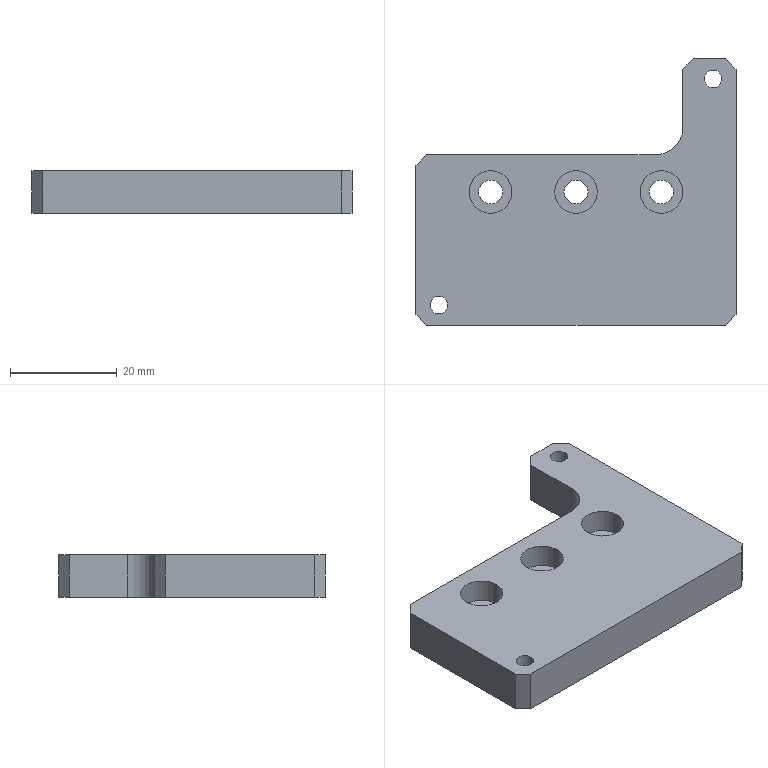Part | SolidWorks | features Chamfer 2, HoleWzd 2, Extrusion 1, Fillet 1, ICE 1 | 1 solid | 33 faces | box 60 x 50 x 8 mm | volume 15791 mm3 | cylinder 17 | plane 16 | commonest cylinder face diameters 4.5 x6 8 x6 3.3 x4 10 x1
STEP:
#1=CARTESIAN_POINT('',(2.65,3.8,0.));
#2=VERTEX_POINT('',#1);
#3=CARTESIAN_POINT('',(5.95,3.8,0.));
#4=VERTEX_POINT('',#3);
#5=CARTESIAN_POINT('',(4.3,3.8,0.));
#6=DIRECTION('',(0.,0.,1.));
#7=DIRECTION('',(1.,0.,0.));
#8=AXIS2_PLACEMENT_3D('',#5,#6,#7);
#9=CIRCLE('',#8,1.65);
#10=EDGE_CURVE('',#2,#4,#9,.T.);
#11=ORIENTED_EDGE('',*,*,#10,.F.);
#12=CARTESIAN_POINT('',(2.65,3.8,8.));
#13=VERTEX_POINT('',#12);
#14=CARTESIAN_POINT('',(2.65,3.8,8.));
#15=DIRECTION('',(0.,0.,1.));
#16=VECTOR('',#15,1000.);
#17=LINE('',#14,#16);
#18=EDGE_CURVE('',#2,#13,#17,.T.);
#19=ORIENTED_EDGE('',*,*,#18,.T.);
#20=CARTESIAN_POINT('',(5.95,3.8,8.));
#21=VERTEX_POINT('',#20);
#22=CARTESIAN_POINT('',(4.3,3.8,8.));
#23=DIRECTION('',(0.,0.,1.));
#24=DIRECTION('',(1.,0.,0.));
#25=AXIS2_PLACEMENT_3D('',#22,#23,#24);
#26=CIRCLE('',#25,1.65);
#27=EDGE_CURVE('',#13,#21,#26,.T.);
#28=ORIENTED_EDGE('',*,*,#27,.T.);
#29=CARTESIAN_POINT('',(5.95,3.8,8.));
#30=DIRECTION('',(0.,0.,1.));
#31=VECTOR('',#30,1000.);
#32=LINE('',#29,#31);
#33=EDGE_CURVE('',#4,#21,#32,.T.);
#34=ORIENTED_EDGE('',*,*,#33,.F.);
#35=EDGE_LOOP('',(#11,#19,#28,#34));
#36=FACE_OUTER_BOUND('',#35,.T.);
#37=CARTESIAN_POINT('',(4.3,3.8,8.));
#38=DIRECTION('',(0.,0.,1.));
#39=DIRECTION('',(1.,0.,0.));
#40=AXIS2_PLACEMENT_3D('',#37,#38,#39);
#41=CYLINDRICAL_SURFACE('',#40,1.65);
#42=ADVANCED_FACE('',(#36),#41,.F.);
#43=CARTESIAN_POINT('',(54.05,46.2,0.));
#44=VERTEX_POINT('',#43);
#45=CARTESIAN_POINT('',(57.35,46.2,0.));
#46=VERTEX_POINT('',#45);
#47=CARTESIAN_POINT('',(55.7,46.2,0.));
#48=DIRECTION('',(0.,0.,1.));
#49=DIRECTION('',(1.,0.,0.));
#50=AXIS2_PLACEMENT_3D('',#47,#48,#49);
#51=CIRCLE('',#50,1.65);
#52=EDGE_CURVE('',#44,#46,#51,.T.);
#53=ORIENTED_EDGE('',*,*,#52,.F.);
#54=CARTESIAN_POINT('',(54.05,46.2,8.));
#55=VERTEX_POINT('',#54);
#56=CARTESIAN_POINT('',(54.05,46.2,8.));
#57=DIRECTION('',(0.,0.,1.));
#58=VECTOR('',#57,1000.);
#59=LINE('',#56,#58);
#60=EDGE_CURVE('',#44,#55,#59,.T.);
#61=ORIENTED_EDGE('',*,*,#60,.T.);
#62=CARTESIAN_POINT('',(57.35,46.2,8.));
#63=VERTEX_POINT('',#62);
#64=CARTESIAN_POINT('',(55.7,46.2,8.));
#65=DIRECTION('',(0.,0.,1.));
#66=DIRECTION('',(1.,0.,0.));
#67=AXIS2_PLACEMENT_3D('',#64,#65,#66);
#68=CIRCLE('',#67,1.65);
#69=EDGE_CURVE('',#55,#63,#68,.T.);
#70=ORIENTED_EDGE('',*,*,#69,.T.);
#71=CARTESIAN_POINT('',(57.35,46.2,8.));
#72=DIRECTION('',(0.,0.,1.));
#73=VECTOR('',#72,1000.);
#74=LINE('',#71,#73);
#75=EDGE_CURVE('',#46,#63,#74,.T.);
#76=ORIENTED_EDGE('',*,*,#75,.F.);
#77=EDGE_LOOP('',(#53,#61,#70,#76));
#78=FACE_OUTER_BOUND('',#77,.T.);
#79=CARTESIAN_POINT('',(55.7,46.2,8.));
#80=DIRECTION('',(0.,0.,1.));
#81=DIRECTION('',(1.,0.,0.));
#82=AXIS2_PLACEMENT_3D('',#79,#80,#81);
#83=CYLINDRICAL_SURFACE('',#82,1.65);
#84=ADVANCED_FACE('',(#78),#83,.F.);
#85=CARTESIAN_POINT('',(26.,25.,3.6));
#86=VERTEX_POINT('',#85);
#87=CARTESIAN_POINT('',(34.,25.,3.6));
#88=VERTEX_POINT('',#87);
#89=CARTESIAN_POINT('',(30.,25.,3.6));
#90=DIRECTION('',(0.,0.,1.));
#91=DIRECTION('',(1.,0.,0.));
#92=AXIS2_PLACEMENT_3D('',#89,#90,#91);
#93=CIRCLE('',#92,4.);
#94=EDGE_CURVE('',#86,#88,#93,.T.);
#95=ORIENTED_EDGE('',*,*,#94,.F.);
#96=CARTESIAN_POINT('',(26.,25.,8.));
#97=VERTEX_POINT('',#96);
#98=CARTESIAN_POINT('',(26.,25.,8.));
#99=DIRECTION('',(0.,0.,1.));
#100=VECTOR('',#99,1000.);
#101=LINE('',#98,#100);
#102=EDGE_CURVE('',#86,#97,#101,.T.);
#103=ORIENTED_EDGE('',*,*,#102,.T.);
#104=CARTESIAN_POINT('',(34.,25.,8.));
#105=VERTEX_POINT('',#104);
#106=CARTESIAN_POINT('',(30.,25.,8.));
#107=DIRECTION('',(0.,0.,1.));
#108=DIRECTION('',(1.,0.,0.));
#109=AXIS2_PLACEMENT_3D('',#106,#107,#108);
#110=CIRCLE('',#109,4.);
#111=EDGE_CURVE('',#97,#105,#110,.T.);
#112=ORIENTED_EDGE('',*,*,#111,.T.);
#113=CARTESIAN_POINT('',(34.,25.,8.));
#114=DIRECTION('',(0.,0.,1.));
#115=VECTOR('',#114,1000.);
#116=LINE('',#113,#115);
#117=EDGE_CURVE('',#88,#105,#116,.T.);
#118=ORIENTED_EDGE('',*,*,#117,.F.);
#119=EDGE_LOOP('',(#95,#103,#112,#118));
#120=FACE_OUTER_BOUND('',#119,.T.);
#121=CARTESIAN_POINT('',(30.,25.,8.));
#122=DIRECTION('',(0.,0.,1.));
#123=DIRECTION('',(1.,0.,0.));
#124=AXIS2_PLACEMENT_3D('',#121,#122,#123);
#125=CYLINDRICAL_SURFACE('',#124,4.);
#126=ADVANCED_FACE('',(#120),#125,.F.);
#127=CARTESIAN_POINT('',(27.75,25.,0.));
#128=VERTEX_POINT('',#127);
#129=CARTESIAN_POINT('',(32.25,25.,0.));
#130=VERTEX_POINT('',#129);
#131=CARTESIAN_POINT('',(30.,25.,0.));
#132=DIRECTION('',(0.,0.,1.));
#133=DIRECTION('',(1.,0.,0.));
#134=AXIS2_PLACEMENT_3D('',#131,#132,#133);
#135=CIRCLE('',#134,2.25);
#136=EDGE_CURVE('',#128,#130,#135,.T.);
#137=ORIENTED_EDGE('',*,*,#136,.F.);
#138=CARTESIAN_POINT('',(27.75,25.,3.6));
#139=VERTEX_POINT('',#138);
#140=CARTESIAN_POINT('',(27.75,25.,8.));
#141=DIRECTION('',(0.,0.,1.));
#142=VECTOR('',#141,1000.);
#143=LINE('',#140,#142);
#144=EDGE_CURVE('',#128,#139,#143,.T.);
#145=ORIENTED_EDGE('',*,*,#144,.T.);
#146=CARTESIAN_POINT('',(32.25,25.,3.6));
#147=VERTEX_POINT('',#146);
#148=CARTESIAN_POINT('',(30.,25.,3.6));
#149=DIRECTION('',(0.,0.,1.));
#150=DIRECTION('',(1.,0.,0.));
#151=AXIS2_PLACEMENT_3D('',#148,#149,#150);
#152=CIRCLE('',#151,2.25);
#153=EDGE_CURVE('',#139,#147,#152,.T.);
#154=ORIENTED_EDGE('',*,*,#153,.T.);
#155=CARTESIAN_POINT('',(32.25,25.,8.));
#156=DIRECTION('',(0.,0.,1.));
#157=VECTOR('',#156,1000.);
#158=LINE('',#155,#157);
#159=EDGE_CURVE('',#130,#147,#158,.T.);
#160=ORIENTED_EDGE('',*,*,#159,.F.);
#161=EDGE_LOOP('',(#137,#145,#154,#160));
#162=FACE_OUTER_BOUND('',#161,.T.);
#163=CARTESIAN_POINT('',(30.,25.,8.));
#164=DIRECTION('',(0.,0.,1.));
#165=DIRECTION('',(1.,0.,0.));
#166=AXIS2_PLACEMENT_3D('',#163,#164,#165);
#167=CYLINDRICAL_SURFACE('',#166,2.25);
#168=ADVANCED_FACE('',(#162),#167,.F.);
#169=CARTESIAN_POINT('',(10.,25.,3.6));
#170=VERTEX_POINT('',#169);
#171=CARTESIAN_POINT('',(18.,25.,3.6));
#172=VERTEX_POINT('',#171);
#173=CARTESIAN_POINT('',(14.,25.,3.6));
#174=DIRECTION('',(0.,0.,1.));
#175=DIRECTION('',(1.,0.,0.));
#176=AXIS2_PLACEMENT_3D('',#173,#174,#175);
#177=CIRCLE('',#176,4.);
#178=EDGE_CURVE('',#170,#172,#177,.T.);
#179=ORIENTED_EDGE('',*,*,#178,.F.);
#180=CARTESIAN_POINT('',(10.,25.,8.));
#181=VERTEX_POINT('',#180);
#182=CARTESIAN_POINT('',(10.,25.,8.));
#183=DIRECTION('',(0.,0.,1.));
#184=VECTOR('',#183,1000.);
#185=LINE('',#182,#184);
#186=EDGE_CURVE('',#170,#181,#185,.T.);
#187=ORIENTED_EDGE('',*,*,#186,.T.);
#188=CARTESIAN_POINT('',(18.,25.,8.));
#189=VERTEX_POINT('',#188);
#190=CARTESIAN_POINT('',(14.,25.,8.));
#191=DIRECTION('',(0.,0.,1.));
#192=DIRECTION('',(1.,0.,0.));
#193=AXIS2_PLACEMENT_3D('',#190,#191,#192);
#194=CIRCLE('',#193,4.);
#195=EDGE_CURVE('',#181,#189,#194,.T.);
#196=ORIENTED_EDGE('',*,*,#195,.T.);
#197=CARTESIAN_POINT('',(18.,25.,8.));
#198=DIRECTION('',(0.,0.,1.));
#199=VECTOR('',#198,1000.);
#200=LINE('',#197,#199);
#201=EDGE_CURVE('',#172,#189,#200,.T.);
#202=ORIENTED_EDGE('',*,*,#201,.F.);
#203=EDGE_LOOP('',(#179,#187,#196,#202));
#204=FACE_OUTER_BOUND('',#203,.T.);
#205=CARTESIAN_POINT('',(14.,25.,8.));
#206=DIRECTION('',(0.,0.,1.));
#207=DIRECTION('',(1.,0.,0.));
#208=AXIS2_PLACEMENT_3D('',#205,#206,#207);
#209=CYLINDRICAL_SURFACE('',#208,4.);
#210=ADVANCED_FACE('',(#204),#209,.F.);
#211=CARTESIAN_POINT('',(11.75,25.,0.));
#212=VERTEX_POINT('',#211);
#213=CARTESIAN_POINT('',(16.25,25.,0.));
#214=VERTEX_POINT('',#213);
#215=CARTESIAN_POINT('',(14.,25.,0.));
#216=DIRECTION('',(0.,0.,1.));
#217=DIRECTION('',(1.,0.,0.));
#218=AXIS2_PLACEMENT_3D('',#215,#216,#217);
#219=CIRCLE('',#218,2.25);
#220=EDGE_CURVE('',#212,#214,#219,.T.);
#221=ORIENTED_EDGE('',*,*,#220,.F.);
#222=CARTESIAN_POINT('',(11.75,25.,3.6));
#223=VERTEX_POINT('',#222);
#224=CARTESIAN_POINT('',(11.75,25.,8.));
#225=DIRECTION('',(0.,0.,1.));
#226=VECTOR('',#225,1000.);
#227=LINE('',#224,#226);
#228=EDGE_CURVE('',#212,#223,#227,.T.);
#229=ORIENTED_EDGE('',*,*,#228,.T.);
#230=CARTESIAN_POINT('',(16.25,25.,3.6));
#231=VERTEX_POINT('',#230);
#232=CARTESIAN_POINT('',(14.,25.,3.6));
#233=DIRECTION('',(0.,0.,1.));
#234=DIRECTION('',(1.,0.,0.));
#235=AXIS2_PLACEMENT_3D('',#232,#233,#234);
#236=CIRCLE('',#235,2.25);
#237=EDGE_CURVE('',#223,#231,#236,.T.);
#238=ORIENTED_EDGE('',*,*,#237,.T.);
#239=CARTESIAN_POINT('',(16.25,25.,8.));
#240=DIRECTION('',(0.,0.,1.));
#241=VECTOR('',#240,1000.);
#242=LINE('',#239,#241);
#243=EDGE_CURVE('',#214,#231,#242,.T.);
#244=ORIENTED_EDGE('',*,*,#243,.F.);
#245=EDGE_LOOP('',(#221,#229,#238,#244));
#246=FACE_OUTER_BOUND('',#245,.T.);
#247=CARTESIAN_POINT('',(14.,25.,8.));
#248=DIRECTION('',(0.,0.,1.));
#249=DIRECTION('',(1.,0.,0.));
#250=AXIS2_PLACEMENT_3D('',#247,#248,#249);
#251=CYLINDRICAL_SURFACE('',#250,2.25);
#252=ADVANCED_FACE('',(#246),#251,.F.);
#253=CARTESIAN_POINT('',(42.,25.,3.6));
#254=VERTEX_POINT('',#253);
#255=CARTESIAN_POINT('',(50.,25.,3.6));
#256=VERTEX_POINT('',#255);
#257=CARTESIAN_POINT('',(46.,25.,3.6));
#258=DIRECTION('',(0.,0.,1.));
#259=DIRECTION('',(1.,0.,0.));
#260=AXIS2_PLACEMENT_3D('',#257,#258,#259);
#261=CIRCLE('',#260,4.);
#262=EDGE_CURVE('',#254,#256,#261,.T.);
#263=ORIENTED_EDGE('',*,*,#262,.F.);
#264=CARTESIAN_POINT('',(42.,25.,8.));
#265=VERTEX_POINT('',#264);
#266=CARTESIAN_POINT('',(42.,25.,8.));
#267=DIRECTION('',(0.,0.,1.));
#268=VECTOR('',#267,1000.);
#269=LINE('',#266,#268);
#270=EDGE_CURVE('',#254,#265,#269,.T.);
#271=ORIENTED_EDGE('',*,*,#270,.T.);
#272=CARTESIAN_POINT('',(50.,25.,8.));
#273=VERTEX_POINT('',#272);
#274=CARTESIAN_POINT('',(46.,25.,8.));
#275=DIRECTION('',(0.,0.,1.));
#276=DIRECTION('',(1.,0.,0.));
#277=AXIS2_PLACEMENT_3D('',#274,#275,#276);
#278=CIRCLE('',#277,4.);
#279=EDGE_CURVE('',#265,#273,#278,.T.);
#280=ORIENTED_EDGE('',*,*,#279,.T.);
#281=CARTESIAN_POINT('',(50.,25.,8.));
#282=DIRECTION('',(0.,0.,1.));
#283=VECTOR('',#282,1000.);
#284=LINE('',#281,#283);
#285=EDGE_CURVE('',#256,#273,#284,.T.);
#286=ORIENTED_EDGE('',*,*,#285,.F.);
#287=EDGE_LOOP('',(#263,#271,#280,#286));
#288=FACE_OUTER_BOUND('',#287,.T.);
#289=CARTESIAN_POINT('',(46.,25.,8.));
#290=DIRECTION('',(0.,0.,1.));
#291=DIRECTION('',(1.,0.,0.));
#292=AXIS2_PLACEMENT_3D('',#289,#290,#291);
#293=CYLINDRICAL_SURFACE('',#292,4.);
#294=ADVANCED_FACE('',(#288),#293,.F.);
#295=CARTESIAN_POINT('',(43.75,25.,0.));
#296=VERTEX_POINT('',#295);
#297=CARTESIAN_POINT('',(48.25,25.,0.));
#298=VERTEX_POINT('',#297);
#299=CARTESIAN_POINT('',(46.,25.,0.));
#300=DIRECTION('',(0.,0.,1.));
#301=DIRECTION('',(1.,0.,0.));
#302=AXIS2_PLACEMENT_3D('',#299,#300,#301);
#303=CIRCLE('',#302,2.25);
#304=EDGE_CURVE('',#296,#298,#303,.T.);
#305=ORIENTED_EDGE('',*,*,#304,.F.);
#306=CARTESIAN_POINT('',(43.75,25.,3.6));
#307=VERTEX_POINT('',#306);
#308=CARTESIAN_POINT('',(43.75,25.,8.));
#309=DIRECTION('',(0.,0.,1.));
#310=VECTOR('',#309,1000.);
#311=LINE('',#308,#310);
#312=EDGE_CURVE('',#296,#307,#311,.T.);
#313=ORIENTED_EDGE('',*,*,#312,.T.);
#314=CARTESIAN_POINT('',(48.25,25.,3.6));
#315=VERTEX_POINT('',#314);
#316=CARTESIAN_POINT('',(46.,25.,3.6));
#317=DIRECTION('',(0.,0.,1.));
#318=DIRECTION('',(1.,0.,0.));
#319=AXIS2_PLACEMENT_3D('',#316,#317,#318);
#320=CIRCLE('',#319,2.25);
#321=EDGE_CURVE('',#307,#315,#320,.T.);
#322=ORIENTED_EDGE('',*,*,#321,.T.);
#323=CARTESIAN_POINT('',(48.25,25.,8.));
#324=DIRECTION('',(0.,0.,1.));
#325=VECTOR('',#324,1000.);
#326=LINE('',#323,#325);
#327=EDGE_CURVE('',#298,#315,#326,.T.);
#328=ORIENTED_EDGE('',*,*,#327,.F.);
#329=EDGE_LOOP('',(#305,#313,#322,#328));
#330=FACE_OUTER_BOUND('',#329,.T.);
#331=CARTESIAN_POINT('',(46.,25.,8.));
#332=DIRECTION('',(0.,0.,1.));
#333=DIRECTION('',(1.,0.,0.));
#334=AXIS2_PLACEMENT_3D('',#331,#332,#333);
#335=CYLINDRICAL_SURFACE('',#334,2.25);
#336=ADVANCED_FACE('',(#330),#335,.F.);
#337=CARTESIAN_POINT('',(0.,30.,8.));
#338=VERTEX_POINT('',#337);
#339=CARTESIAN_POINT('',(0.,2.,8.));
#340=VERTEX_POINT('',#339);
#341=CARTESIAN_POINT('',(0.,0.,8.));
#342=DIRECTION('',(0.,-1.,0.));
#343=VECTOR('',#342,1000.);
#344=LINE('',#341,#343);
#345=EDGE_CURVE('',#338,#340,#344,.T.);
#346=ORIENTED_EDGE('',*,*,#345,.F.);
#347=CARTESIAN_POINT('',(0.,30.,0.));
#348=VERTEX_POINT('',#347);
#349=CARTESIAN_POINT('',(0.,30.,8.));
#350=DIRECTION('',(0.,0.,-1.));
#351=VECTOR('',#350,1000.);
#352=LINE('',#349,#351);
#353=EDGE_CURVE('',#338,#348,#352,.T.);
#354=ORIENTED_EDGE('',*,*,#353,.T.);
#355=CARTESIAN_POINT('',(0.,2.,0.));
#356=VERTEX_POINT('',#355);
#357=CARTESIAN_POINT('',(0.,0.,0.));
#358=DIRECTION('',(0.,-1.,0.));
#359=VECTOR('',#358,1000.);
#360=LINE('',#357,#359);
#361=EDGE_CURVE('',#348,#356,#360,.T.);
#362=ORIENTED_EDGE('',*,*,#361,.T.);
#363=CARTESIAN_POINT('',(0.,2.,8.));
#364=DIRECTION('',(0.,0.,1.));
#365=VECTOR('',#364,1000.);
#366=LINE('',#363,#365);
#367=EDGE_CURVE('',#356,#340,#366,.T.);
#368=ORIENTED_EDGE('',*,*,#367,.T.);
#369=EDGE_LOOP('',(#346,#354,#362,#368));
#370=FACE_OUTER_BOUND('',#369,.T.);
#371=CARTESIAN_POINT('',(0.,0.,8.));
#372=DIRECTION('',(1.,0.,0.));
#373=DIRECTION('',(0.,0.,-1.));
#374=AXIS2_PLACEMENT_3D('',#371,#372,#373);
#375=PLANE('',#374);
#376=ADVANCED_FACE('',(#370),#375,.F.);
#377=CARTESIAN_POINT('',(2.,0.,0.));
#378=VERTEX_POINT('',#377);
#379=CARTESIAN_POINT('',(58.,0.,0.));
#380=VERTEX_POINT('',#379);
#381=CARTESIAN_POINT('',(0.,0.,0.));
#382=DIRECTION('',(1.,0.,0.));
#383=VECTOR('',#382,1000.);
#384=LINE('',#381,#383);
#385=EDGE_CURVE('',#378,#380,#384,.T.);
#386=ORIENTED_EDGE('',*,*,#385,.T.);
#387=CARTESIAN_POINT('',(58.,0.,8.));
#388=VERTEX_POINT('',#387);
#389=CARTESIAN_POINT('',(58.,0.,8.));
#390=DIRECTION('',(0.,0.,1.));
#391=VECTOR('',#390,1000.);
#392=LINE('',#389,#391);
#393=EDGE_CURVE('',#380,#388,#392,.T.);
#394=ORIENTED_EDGE('',*,*,#393,.T.);
#395=CARTESIAN_POINT('',(2.,0.,8.));
#396=VERTEX_POINT('',#395);
#397=CARTESIAN_POINT('',(0.,0.,8.));
#398=DIRECTION('',(1.,0.,0.));
#399=VECTOR('',#398,1000.);
#400=LINE('',#397,#399);
#401=EDGE_CURVE('',#396,#388,#400,.T.);
#402=ORIENTED_EDGE('',*,*,#401,.F.);
#403=CARTESIAN_POINT('',(2.,0.,8.));
#404=DIRECTION('',(0.,0.,-1.));
#405=VECTOR('',#404,1000.);
#406=LINE('',#403,#405);
#407=EDGE_CURVE('',#396,#378,#406,.T.);
#408=ORIENTED_EDGE('',*,*,#407,.T.);
#409=EDGE_LOOP('',(#386,#394,#402,#408));
#410=FACE_OUTER_BOUND('',#409,.T.);
#411=CARTESIAN_POINT('',(0.,0.,8.));
#412=DIRECTION('',(0.,1.,0.));
#413=DIRECTION('',(0.,0.,1.));
#414=AXIS2_PLACEMENT_3D('',#411,#412,#413);
#415=PLANE('',#414);
#416=ADVANCED_FACE('',(#410),#415,.F.);
#417=CARTESIAN_POINT('',(60.,2.,0.));
#418=VERTEX_POINT('',#417);
#419=CARTESIAN_POINT('',(60.,48.,0.));
#420=VERTEX_POINT('',#419);
#421=CARTESIAN_POINT('',(60.,0.,0.));
#422=DIRECTION('',(0.,1.,0.));
#423=VECTOR('',#422,1000.);
#424=LINE('',#421,#423);
#425=EDGE_CURVE('',#418,#420,#424,.T.);
#426=ORIENTED_EDGE('',*,*,#425,.T.);
#427=CARTESIAN_POINT('',(60.,48.,8.));
#428=VERTEX_POINT('',#427);
#429=CARTESIAN_POINT('',(60.,48.,8.));
#430=DIRECTION('',(0.,0.,1.));
#431=VECTOR('',#430,1000.);
#432=LINE('',#429,#431);
#433=EDGE_CURVE('',#420,#428,#432,.T.);
#434=ORIENTED_EDGE('',*,*,#433,.T.);
#435=CARTESIAN_POINT('',(60.,2.,8.));
#436=VERTEX_POINT('',#435);
#437=CARTESIAN_POINT('',(60.,0.,8.));
#438=DIRECTION('',(0.,1.,0.));
#439=VECTOR('',#438,1000.);
#440=LINE('',#437,#439);
#441=EDGE_CURVE('',#436,#428,#440,.T.);
#442=ORIENTED_EDGE('',*,*,#441,.F.);
#443=CARTESIAN_POINT('',(60.,2.,8.));
#444=DIRECTION('',(0.,0.,-1.));
#445=VECTOR('',#444,1000.);
#446=LINE('',#443,#445);
#447=EDGE_CURVE('',#436,#418,#446,.T.);
#448=ORIENTED_EDGE('',*,*,#447,.T.);
#449=EDGE_LOOP('',(#426,#434,#442,#448));
#450=FACE_OUTER_BOUND('',#449,.T.);
#451=CARTESIAN_POINT('',(60.,0.,8.));
#452=DIRECTION('',(-1.,0.,0.));
#453=DIRECTION('',(0.,0.,1.));
#454=AXIS2_PLACEMENT_3D('',#451,#452,#453);
#455=PLANE('',#454);
#456=ADVANCED_FACE('',(#450),#455,.F.);
#457=CARTESIAN_POINT('',(58.,50.,0.));
#458=VERTEX_POINT('',#457);
#459=CARTESIAN_POINT('',(52.,50.,0.));
#460=VERTEX_POINT('',#459);
#461=CARTESIAN_POINT('',(0.,50.,0.));
#462=DIRECTION('',(-1.,0.,0.));
#463=VECTOR('',#462,1000.);
#464=LINE('',#461,#463);
#465=EDGE_CURVE('',#458,#460,#464,.T.);
#466=ORIENTED_EDGE('',*,*,#465,.T.);
#467=CARTESIAN_POINT('',(52.,50.,8.));
#468=VERTEX_POINT('',#467);
#469=CARTESIAN_POINT('',(52.,50.,8.));
#470=DIRECTION('',(0.,0.,1.));
#471=VECTOR('',#470,1000.);
#472=LINE('',#469,#471);
#473=EDGE_CURVE('',#460,#468,#472,.T.);
#474=ORIENTED_EDGE('',*,*,#473,.T.);
#475=CARTESIAN_POINT('',(58.,50.,8.));
#476=VERTEX_POINT('',#475);
#477=CARTESIAN_POINT('',(0.,50.,8.));
#478=DIRECTION('',(-1.,0.,0.));
#479=VECTOR('',#478,1000.);
#480=LINE('',#477,#479);
#481=EDGE_CURVE('',#476,#468,#480,.T.);
#482=ORIENTED_EDGE('',*,*,#481,.F.);
#483=CARTESIAN_POINT('',(58.,50.,8.));
#484=DIRECTION('',(0.,0.,-1.));
#485=VECTOR('',#484,1000.);
#486=LINE('',#483,#485);
#487=EDGE_CURVE('',#476,#458,#486,.T.);
#488=ORIENTED_EDGE('',*,*,#487,.T.);
#489=EDGE_LOOP('',(#466,#474,#482,#488));
#490=FACE_OUTER_BOUND('',#489,.T.);
#491=CARTESIAN_POINT('',(0.,50.,8.));
#492=DIRECTION('',(0.,-1.,0.));
#493=DIRECTION('',(0.,0.,-1.));
#494=AXIS2_PLACEMENT_3D('',#491,#492,#493);
#495=PLANE('',#494);
#496=ADVANCED_FACE('',(#490),#495,.F.);
#497=CARTESIAN_POINT('',(4.3,3.8,8.));
#498=DIRECTION('',(0.,0.,1.));
#499=DIRECTION('',(1.,0.,0.));
#500=AXIS2_PLACEMENT_3D('',#497,#498,#499);
#501=CIRCLE('',#500,1.65);
#502=EDGE_CURVE('',#21,#13,#501,.T.);
#503=ORIENTED_EDGE('',*,*,#502,.F.);
#504=ORIENTED_EDGE('',*,*,#27,.F.);
#505=EDGE_LOOP('',(#503,#504));
#506=FACE_BOUND('',#505,.T.);
#507=CARTESIAN_POINT('',(55.7,46.2,8.));
#508=DIRECTION('',(0.,0.,1.));
#509=DIRECTION('',(1.,0.,0.));
#510=AXIS2_PLACEMENT_3D('',#507,#508,#509);
#511=CIRCLE('',#510,1.65);
#512=EDGE_CURVE('',#63,#55,#511,.T.);
#513=ORIENTED_EDGE('',*,*,#512,.F.);
#514=ORIENTED_EDGE('',*,*,#69,.F.);
#515=EDGE_LOOP('',(#513,#514));
#516=FACE_BOUND('',#515,.T.);
#517=CARTESIAN_POINT('',(30.,25.,8.));
#518=DIRECTION('',(0.,0.,1.));
#519=DIRECTION('',(1.,0.,0.));
#520=AXIS2_PLACEMENT_3D('',#517,#518,#519);
#521=CIRCLE('',#520,4.);
#522=EDGE_CURVE('',#105,#97,#521,.T.);
#523=ORIENTED_EDGE('',*,*,#522,.F.);
#524=ORIENTED_EDGE('',*,*,#111,.F.);
#525=EDGE_LOOP('',(#523,#524));
#526=FACE_BOUND('',#525,.T.);
#527=CARTESIAN_POINT('',(14.,25.,8.));
#528=DIRECTION('',(0.,0.,1.));
#529=DIRECTION('',(1.,0.,0.));
#530=AXIS2_PLACEMENT_3D('',#527,#528,#529);
#531=CIRCLE('',#530,4.);
#532=EDGE_CURVE('',#189,#181,#531,.T.);
#533=ORIENTED_EDGE('',*,*,#532,.F.);
#534=ORIENTED_EDGE('',*,*,#195,.F.);
#535=EDGE_LOOP('',(#533,#534));
#536=FACE_BOUND('',#535,.T.);
#537=CARTESIAN_POINT('',(46.,25.,8.));
#538=DIRECTION('',(0.,0.,1.));
#539=DIRECTION('',(1.,0.,0.));
#540=AXIS2_PLACEMENT_3D('',#537,#538,#539);
#541=CIRCLE('',#540,4.);
#542=EDGE_CURVE('',#273,#265,#541,.T.);
#543=ORIENTED_EDGE('',*,*,#542,.F.);
#544=ORIENTED_EDGE('',*,*,#279,.F.);
#545=EDGE_LOOP('',(#543,#544));
#546=FACE_BOUND('',#545,.T.);
#547=CARTESIAN_POINT('',(50.,48.,8.));
#548=VERTEX_POINT('',#547);
#549=CARTESIAN_POINT('',(50.,37.,8.));
#550=VERTEX_POINT('',#549);
#551=CARTESIAN_POINT('',(50.,32.,8.));
#552=DIRECTION('',(0.,-1.,0.));
#553=VECTOR('',#552,1000.);
#554=LINE('',#551,#553);
#555=EDGE_CURVE('',#548,#550,#554,.T.);
#556=ORIENTED_EDGE('',*,*,#555,.T.);
#557=CARTESIAN_POINT('',(45.,32.,8.));
#558=VERTEX_POINT('',#557);
#559=CARTESIAN_POINT('',(45.,37.,8.));
#560=DIRECTION('',(0.,0.,-1.));
#561=DIRECTION('',(-1.,0.,0.));
#562=AXIS2_PLACEMENT_3D('',#559,#560,#561);
#563=CIRCLE('',#562,5.);
#564=EDGE_CURVE('',#550,#558,#563,.T.);
#565=ORIENTED_EDGE('',*,*,#564,.T.);
#566=CARTESIAN_POINT('',(2.,32.,8.));
#567=VERTEX_POINT('',#566);
#568=CARTESIAN_POINT('',(50.,32.,8.));
#569=DIRECTION('',(-1.,0.,0.));
#570=VECTOR('',#569,1000.);
#571=LINE('',#568,#570);
#572=EDGE_CURVE('',#558,#567,#571,.T.);
#573=ORIENTED_EDGE('',*,*,#572,.T.);
#574=CARTESIAN_POINT('',(0.,30.,8.));
#575=DIRECTION('',(-0.7071,-0.7071,0.));
#576=VECTOR('',#575,1000.);
#577=LINE('',#574,#576);
#578=EDGE_CURVE('',#567,#338,#577,.T.);
#579=ORIENTED_EDGE('',*,*,#578,.T.);
#580=ORIENTED_EDGE('',*,*,#345,.T.);
#581=CARTESIAN_POINT('',(2.,0.,8.));
#582=DIRECTION('',(0.7071,-0.7071,0.));
#583=VECTOR('',#582,1000.);
#584=LINE('',#581,#583);
#585=EDGE_CURVE('',#340,#396,#584,.T.);
#586=ORIENTED_EDGE('',*,*,#585,.T.);
#587=ORIENTED_EDGE('',*,*,#401,.T.);
#588=CARTESIAN_POINT('',(60.,2.,8.));
#589=DIRECTION('',(0.7071,0.7071,0.));
#590=VECTOR('',#589,1000.);
#591=LINE('',#588,#590);
#592=EDGE_CURVE('',#388,#436,#591,.T.);
#593=ORIENTED_EDGE('',*,*,#592,.T.);
#594=ORIENTED_EDGE('',*,*,#441,.T.);
#595=CARTESIAN_POINT('',(58.,50.,8.));
#596=DIRECTION('',(-0.7071,0.7071,0.));
#597=VECTOR('',#596,1000.);
#598=LINE('',#595,#597);
#599=EDGE_CURVE('',#428,#476,#598,.T.);
#600=ORIENTED_EDGE('',*,*,#599,.T.);
#601=ORIENTED_EDGE('',*,*,#481,.T.);
#602=CARTESIAN_POINT('',(50.,48.,8.));
#603=DIRECTION('',(-0.7071,-0.7071,0.));
#604=VECTOR('',#603,1000.);
#605=LINE('',#602,#604);
#606=EDGE_CURVE('',#468,#548,#605,.T.);
#607=ORIENTED_EDGE('',*,*,#606,.T.);
#608=EDGE_LOOP('',(#556,#565,#573,#579,#580,#586,#587,#593,#594,#600,#601,#607));
#609=FACE_OUTER_BOUND('',#608,.T.);
#610=CARTESIAN_POINT('',(0.,0.,8.));
#611=DIRECTION('',(0.,0.,-1.));
#612=DIRECTION('',(-1.,0.,0.));
#613=AXIS2_PLACEMENT_3D('',#610,#611,#612);
#614=PLANE('',#613);
#615=ADVANCED_FACE('',(#506,#516,#526,#536,#546,#609),#614,.F.);
#616=ORIENTED_EDGE('',*,*,#361,.F.);
#617=CARTESIAN_POINT('',(2.,32.,0.));
#618=VERTEX_POINT('',#617);
#619=CARTESIAN_POINT('',(-15.,15.,0.));
#620=DIRECTION('',(0.7071,0.7071,0.));
#621=VECTOR('',#620,1000.);
#622=LINE('',#619,#621);
#623=EDGE_CURVE('',#348,#618,#622,.T.);
#624=ORIENTED_EDGE('',*,*,#623,.T.);
#625=CARTESIAN_POINT('',(45.,32.,0.));
#626=VERTEX_POINT('',#625);
#627=CARTESIAN_POINT('',(50.,32.,0.));
#628=DIRECTION('',(-1.,0.,0.));
#629=VECTOR('',#628,1000.);
#630=LINE('',#627,#629);
#631=EDGE_CURVE('',#626,#618,#630,.T.);
#632=ORIENTED_EDGE('',*,*,#631,.F.);
#633=CARTESIAN_POINT('',(50.,37.,0.));
#634=VERTEX_POINT('',#633);
#635=CARTESIAN_POINT('',(45.,37.,0.));
#636=DIRECTION('',(0.,0.,1.));
#637=DIRECTION('',(-1.,0.,0.));
#638=AXIS2_PLACEMENT_3D('',#635,#636,#637);
#639=CIRCLE('',#638,5.);
#640=EDGE_CURVE('',#626,#634,#639,.T.);
#641=ORIENTED_EDGE('',*,*,#640,.T.);
#642=CARTESIAN_POINT('',(50.,48.,0.));
#643=VERTEX_POINT('',#642);
#644=CARTESIAN_POINT('',(50.,32.,0.));
#645=DIRECTION('',(0.,-1.,0.));
#646=VECTOR('',#645,1000.);
#647=LINE('',#644,#646);
#648=EDGE_CURVE('',#643,#634,#647,.T.);
#649=ORIENTED_EDGE('',*,*,#648,.F.);
#650=CARTESIAN_POINT('',(1.,-1.,0.));
#651=DIRECTION('',(0.7071,0.7071,0.));
#652=VECTOR('',#651,1000.);
#653=LINE('',#650,#652);
#654=EDGE_CURVE('',#643,#460,#653,.T.);
#655=ORIENTED_EDGE('',*,*,#654,.T.);
#656=ORIENTED_EDGE('',*,*,#465,.F.);
#657=CARTESIAN_POINT('',(54.,54.,0.));
#658=DIRECTION('',(0.7071,-0.7071,0.));
#659=VECTOR('',#658,1000.);
#660=LINE('',#657,#659);
#661=EDGE_CURVE('',#458,#420,#660,.T.);
#662=ORIENTED_EDGE('',*,*,#661,.T.);
#663=ORIENTED_EDGE('',*,*,#425,.F.);
#664=CARTESIAN_POINT('',(29.,-29.,0.));
#665=DIRECTION('',(-0.7071,-0.7071,0.));
#666=VECTOR('',#665,1000.);
#667=LINE('',#664,#666);
#668=EDGE_CURVE('',#418,#380,#667,.T.);
#669=ORIENTED_EDGE('',*,*,#668,.T.);
#670=ORIENTED_EDGE('',*,*,#385,.F.);
#671=CARTESIAN_POINT('',(1.,1.,0.));
#672=DIRECTION('',(-0.7071,0.7071,0.));
#673=VECTOR('',#672,1000.);
#674=LINE('',#671,#673);
#675=EDGE_CURVE('',#378,#356,#674,.T.);
#676=ORIENTED_EDGE('',*,*,#675,.T.);
#677=EDGE_LOOP('',(#616,#624,#632,#641,#649,#655,#656,#662,#663,#669,#670,#676));
#678=FACE_OUTER_BOUND('',#677,.T.);
#679=CARTESIAN_POINT('',(4.3,3.8,0.));
#680=DIRECTION('',(0.,0.,1.));
#681=DIRECTION('',(1.,0.,0.));
#682=AXIS2_PLACEMENT_3D('',#679,#680,#681);
#683=CIRCLE('',#682,1.65);
#684=EDGE_CURVE('',#4,#2,#683,.T.);
#685=ORIENTED_EDGE('',*,*,#684,.T.);
#686=ORIENTED_EDGE('',*,*,#10,.T.);
#687=EDGE_LOOP('',(#685,#686));
#688=FACE_BOUND('',#687,.T.);
#689=CARTESIAN_POINT('',(55.7,46.2,0.));
#690=DIRECTION('',(0.,0.,1.));
#691=DIRECTION('',(1.,0.,0.));
#692=AXIS2_PLACEMENT_3D('',#689,#690,#691);
#693=CIRCLE('',#692,1.65);
#694=EDGE_CURVE('',#46,#44,#693,.T.);
#695=ORIENTED_EDGE('',*,*,#694,.T.);
#696=ORIENTED_EDGE('',*,*,#52,.T.);
#697=EDGE_LOOP('',(#695,#696));
#698=FACE_BOUND('',#697,.T.);
#699=CARTESIAN_POINT('',(30.,25.,0.));
#700=DIRECTION('',(0.,0.,1.));
#701=DIRECTION('',(1.,0.,0.));
#702=AXIS2_PLACEMENT_3D('',#699,#700,#701);
#703=CIRCLE('',#702,2.25);
#704=EDGE_CURVE('',#130,#128,#703,.T.);
#705=ORIENTED_EDGE('',*,*,#704,.T.);
#706=ORIENTED_EDGE('',*,*,#136,.T.);
#707=EDGE_LOOP('',(#705,#706));
#708=FACE_BOUND('',#707,.T.);
#709=CARTESIAN_POINT('',(14.,25.,0.));
#710=DIRECTION('',(0.,0.,1.));
#711=DIRECTION('',(1.,0.,0.));
#712=AXIS2_PLACEMENT_3D('',#709,#710,#711);
#713=CIRCLE('',#712,2.25);
#714=EDGE_CURVE('',#214,#212,#713,.T.);
#715=ORIENTED_EDGE('',*,*,#714,.T.);
#716=ORIENTED_EDGE('',*,*,#220,.T.);
#717=EDGE_LOOP('',(#715,#716));
#718=FACE_BOUND('',#717,.T.);
#719=CARTESIAN_POINT('',(46.,25.,0.));
#720=DIRECTION('',(0.,0.,1.));
#721=DIRECTION('',(1.,0.,0.));
#722=AXIS2_PLACEMENT_3D('',#719,#720,#721);
#723=CIRCLE('',#722,2.25);
#724=EDGE_CURVE('',#298,#296,#723,.T.);
#725=ORIENTED_EDGE('',*,*,#724,.T.);
#726=ORIENTED_EDGE('',*,*,#304,.T.);
#727=EDGE_LOOP('',(#725,#726));
#728=FACE_BOUND('',#727,.T.);
#729=CARTESIAN_POINT('',(0.,0.,0.));
#730=DIRECTION('',(0.,0.,-1.));
#731=DIRECTION('',(-1.,0.,0.));
#732=AXIS2_PLACEMENT_3D('',#729,#730,#731);
#733=PLANE('',#732);
#734=ADVANCED_FACE('',(#678,#688,#698,#708,#718,#728),#733,.T.);
#735=ORIENTED_EDGE('',*,*,#312,.F.);
#736=ORIENTED_EDGE('',*,*,#724,.F.);
#737=ORIENTED_EDGE('',*,*,#327,.T.);
#738=CARTESIAN_POINT('',(46.,25.,3.6));
#739=DIRECTION('',(0.,0.,1.));
#740=DIRECTION('',(1.,0.,0.));
#741=AXIS2_PLACEMENT_3D('',#738,#739,#740);
#742=CIRCLE('',#741,2.25);
#743=EDGE_CURVE('',#315,#307,#742,.T.);
#744=ORIENTED_EDGE('',*,*,#743,.T.);
#745=EDGE_LOOP('',(#735,#736,#737,#744));
#746=FACE_OUTER_BOUND('',#745,.T.);
#747=CARTESIAN_POINT('',(46.,25.,8.));
#748=DIRECTION('',(0.,0.,1.));
#749=DIRECTION('',(1.,0.,0.));
#750=AXIS2_PLACEMENT_3D('',#747,#748,#749);
#751=CYLINDRICAL_SURFACE('',#750,2.25);
#752=ADVANCED_FACE('',(#746),#751,.F.);
#753=ORIENTED_EDGE('',*,*,#743,.F.);
#754=ORIENTED_EDGE('',*,*,#321,.F.);
#755=EDGE_LOOP('',(#753,#754));
#756=FACE_BOUND('',#755,.T.);
#757=CARTESIAN_POINT('',(46.,25.,3.6));
#758=DIRECTION('',(0.,0.,1.));
#759=DIRECTION('',(1.,0.,0.));
#760=AXIS2_PLACEMENT_3D('',#757,#758,#759);
#761=CIRCLE('',#760,4.);
#762=EDGE_CURVE('',#256,#254,#761,.T.);
#763=ORIENTED_EDGE('',*,*,#762,.T.);
#764=ORIENTED_EDGE('',*,*,#262,.T.);
#765=EDGE_LOOP('',(#763,#764));
#766=FACE_OUTER_BOUND('',#765,.T.);
#767=CARTESIAN_POINT('',(48.25,25.,3.6));
#768=DIRECTION('',(0.,0.,-1.));
#769=DIRECTION('',(-1.,0.,0.));
#770=AXIS2_PLACEMENT_3D('',#767,#768,#769);
#771=PLANE('',#770);
#772=ADVANCED_FACE('',(#756,#766),#771,.F.);
#773=ORIENTED_EDGE('',*,*,#270,.F.);
#774=ORIENTED_EDGE('',*,*,#762,.F.);
#775=ORIENTED_EDGE('',*,*,#285,.T.);
#776=ORIENTED_EDGE('',*,*,#542,.T.);
#777=EDGE_LOOP('',(#773,#774,#775,#776));
#778=FACE_OUTER_BOUND('',#777,.T.);
#779=CARTESIAN_POINT('',(46.,25.,8.));
#780=DIRECTION('',(0.,0.,1.));
#781=DIRECTION('',(1.,0.,0.));
#782=AXIS2_PLACEMENT_3D('',#779,#780,#781);
#783=CYLINDRICAL_SURFACE('',#782,4.);
#784=ADVANCED_FACE('',(#778),#783,.F.);
#785=ORIENTED_EDGE('',*,*,#228,.F.);
#786=ORIENTED_EDGE('',*,*,#714,.F.);
#787=ORIENTED_EDGE('',*,*,#243,.T.);
#788=CARTESIAN_POINT('',(14.,25.,3.6));
#789=DIRECTION('',(0.,0.,1.));
#790=DIRECTION('',(1.,0.,0.));
#791=AXIS2_PLACEMENT_3D('',#788,#789,#790);
#792=CIRCLE('',#791,2.25);
#793=EDGE_CURVE('',#231,#223,#792,.T.);
#794=ORIENTED_EDGE('',*,*,#793,.T.);
#795=EDGE_LOOP('',(#785,#786,#787,#794));
#796=FACE_OUTER_BOUND('',#795,.T.);
#797=CARTESIAN_POINT('',(14.,25.,8.));
#798=DIRECTION('',(0.,0.,1.));
#799=DIRECTION('',(1.,0.,0.));
#800=AXIS2_PLACEMENT_3D('',#797,#798,#799);
#801=CYLINDRICAL_SURFACE('',#800,2.25);
#802=ADVANCED_FACE('',(#796),#801,.F.);
#803=ORIENTED_EDGE('',*,*,#793,.F.);
#804=ORIENTED_EDGE('',*,*,#237,.F.);
#805=EDGE_LOOP('',(#803,#804));
#806=FACE_BOUND('',#805,.T.);
#807=CARTESIAN_POINT('',(14.,25.,3.6));
#808=DIRECTION('',(0.,0.,1.));
#809=DIRECTION('',(1.,0.,0.));
#810=AXIS2_PLACEMENT_3D('',#807,#808,#809);
#811=CIRCLE('',#810,4.);
#812=EDGE_CURVE('',#172,#170,#811,.T.);
#813=ORIENTED_EDGE('',*,*,#812,.T.);
#814=ORIENTED_EDGE('',*,*,#178,.T.);
#815=EDGE_LOOP('',(#813,#814));
#816=FACE_OUTER_BOUND('',#815,.T.);
#817=CARTESIAN_POINT('',(16.25,25.,3.6));
#818=DIRECTION('',(0.,0.,-1.));
#819=DIRECTION('',(-1.,0.,0.));
#820=AXIS2_PLACEMENT_3D('',#817,#818,#819);
#821=PLANE('',#820);
#822=ADVANCED_FACE('',(#806,#816),#821,.F.);
#823=ORIENTED_EDGE('',*,*,#186,.F.);
#824=ORIENTED_EDGE('',*,*,#812,.F.);
#825=ORIENTED_EDGE('',*,*,#201,.T.);
#826=ORIENTED_EDGE('',*,*,#532,.T.);
#827=EDGE_LOOP('',(#823,#824,#825,#826));
#828=FACE_OUTER_BOUND('',#827,.T.);
#829=CARTESIAN_POINT('',(14.,25.,8.));
#830=DIRECTION('',(0.,0.,1.));
#831=DIRECTION('',(1.,0.,0.));
#832=AXIS2_PLACEMENT_3D('',#829,#830,#831);
#833=CYLINDRICAL_SURFACE('',#832,4.);
#834=ADVANCED_FACE('',(#828),#833,.F.);
#835=ORIENTED_EDGE('',*,*,#144,.F.);
#836=ORIENTED_EDGE('',*,*,#704,.F.);
#837=ORIENTED_EDGE('',*,*,#159,.T.);
#838=CARTESIAN_POINT('',(30.,25.,3.6));
#839=DIRECTION('',(0.,0.,1.));
#840=DIRECTION('',(1.,0.,0.));
#841=AXIS2_PLACEMENT_3D('',#838,#839,#840);
#842=CIRCLE('',#841,2.25);
#843=EDGE_CURVE('',#147,#139,#842,.T.);
#844=ORIENTED_EDGE('',*,*,#843,.T.);
#845=EDGE_LOOP('',(#835,#836,#837,#844));
#846=FACE_OUTER_BOUND('',#845,.T.);
#847=CARTESIAN_POINT('',(30.,25.,8.));
#848=DIRECTION('',(0.,0.,1.));
#849=DIRECTION('',(1.,0.,0.));
#850=AXIS2_PLACEMENT_3D('',#847,#848,#849);
#851=CYLINDRICAL_SURFACE('',#850,2.25);
#852=ADVANCED_FACE('',(#846),#851,.F.);
#853=ORIENTED_EDGE('',*,*,#843,.F.);
#854=ORIENTED_EDGE('',*,*,#153,.F.);
#855=EDGE_LOOP('',(#853,#854));
#856=FACE_BOUND('',#855,.T.);
#857=CARTESIAN_POINT('',(30.,25.,3.6));
#858=DIRECTION('',(0.,0.,1.));
#859=DIRECTION('',(1.,0.,0.));
#860=AXIS2_PLACEMENT_3D('',#857,#858,#859);
#861=CIRCLE('',#860,4.);
#862=EDGE_CURVE('',#88,#86,#861,.T.);
#863=ORIENTED_EDGE('',*,*,#862,.T.);
#864=ORIENTED_EDGE('',*,*,#94,.T.);
#865=EDGE_LOOP('',(#863,#864));
#866=FACE_OUTER_BOUND('',#865,.T.);
#867=CARTESIAN_POINT('',(32.25,25.,3.6));
#868=DIRECTION('',(0.,0.,-1.));
#869=DIRECTION('',(-1.,0.,0.));
#870=AXIS2_PLACEMENT_3D('',#867,#868,#869);
#871=PLANE('',#870);
#872=ADVANCED_FACE('',(#856,#866),#871,.F.);
#873=ORIENTED_EDGE('',*,*,#102,.F.);
#874=ORIENTED_EDGE('',*,*,#862,.F.);
#875=ORIENTED_EDGE('',*,*,#117,.T.);
#876=ORIENTED_EDGE('',*,*,#522,.T.);
#877=EDGE_LOOP('',(#873,#874,#875,#876));
#878=FACE_OUTER_BOUND('',#877,.T.);
#879=CARTESIAN_POINT('',(30.,25.,8.));
#880=DIRECTION('',(0.,0.,1.));
#881=DIRECTION('',(1.,0.,0.));
#882=AXIS2_PLACEMENT_3D('',#879,#880,#881);
#883=CYLINDRICAL_SURFACE('',#882,4.);
#884=ADVANCED_FACE('',(#878),#883,.F.);
#885=ORIENTED_EDGE('',*,*,#60,.F.);
#886=ORIENTED_EDGE('',*,*,#694,.F.);
#887=ORIENTED_EDGE('',*,*,#75,.T.);
#888=ORIENTED_EDGE('',*,*,#512,.T.);
#889=EDGE_LOOP('',(#885,#886,#887,#888));
#890=FACE_OUTER_BOUND('',#889,.T.);
#891=CARTESIAN_POINT('',(55.7,46.2,8.));
#892=DIRECTION('',(0.,0.,1.));
#893=DIRECTION('',(1.,0.,0.));
#894=AXIS2_PLACEMENT_3D('',#891,#892,#893);
#895=CYLINDRICAL_SURFACE('',#894,1.65);
#896=ADVANCED_FACE('',(#890),#895,.F.);
#897=ORIENTED_EDGE('',*,*,#18,.F.);
#898=ORIENTED_EDGE('',*,*,#684,.F.);
#899=ORIENTED_EDGE('',*,*,#33,.T.);
#900=ORIENTED_EDGE('',*,*,#502,.T.);
#901=EDGE_LOOP('',(#897,#898,#899,#900));
#902=FACE_OUTER_BOUND('',#901,.T.);
#903=CARTESIAN_POINT('',(4.3,3.8,8.));
#904=DIRECTION('',(0.,0.,1.));
#905=DIRECTION('',(1.,0.,0.));
#906=AXIS2_PLACEMENT_3D('',#903,#904,#905);
#907=CYLINDRICAL_SURFACE('',#906,1.65);
#908=ADVANCED_FACE('',(#902),#907,.F.);
#909=ORIENTED_EDGE('',*,*,#599,.F.);
#910=ORIENTED_EDGE('',*,*,#433,.F.);
#911=ORIENTED_EDGE('',*,*,#661,.F.);
#912=ORIENTED_EDGE('',*,*,#487,.F.);
#913=EDGE_LOOP('',(#909,#910,#911,#912));
#914=FACE_OUTER_BOUND('',#913,.T.);
#915=CARTESIAN_POINT('',(58.,50.,8.));
#916=DIRECTION('',(-0.7071,-0.7071,0.));
#917=DIRECTION('',(0.,0.,-1.));
#918=AXIS2_PLACEMENT_3D('',#915,#916,#917);
#919=PLANE('',#918);
#920=ADVANCED_FACE('',(#914),#919,.F.);
#921=ORIENTED_EDGE('',*,*,#592,.F.);
#922=ORIENTED_EDGE('',*,*,#393,.F.);
#923=ORIENTED_EDGE('',*,*,#668,.F.);
#924=ORIENTED_EDGE('',*,*,#447,.F.);
#925=EDGE_LOOP('',(#921,#922,#923,#924));
#926=FACE_OUTER_BOUND('',#925,.T.);
#927=CARTESIAN_POINT('',(60.,2.,8.));
#928=DIRECTION('',(-0.7071,0.7071,0.));
#929=DIRECTION('',(0.,0.,-1.));
#930=AXIS2_PLACEMENT_3D('',#927,#928,#929);
#931=PLANE('',#930);
#932=ADVANCED_FACE('',(#926),#931,.F.);
#933=ORIENTED_EDGE('',*,*,#585,.F.);
#934=ORIENTED_EDGE('',*,*,#367,.F.);
#935=ORIENTED_EDGE('',*,*,#675,.F.);
#936=ORIENTED_EDGE('',*,*,#407,.F.);
#937=EDGE_LOOP('',(#933,#934,#935,#936));
#938=FACE_OUTER_BOUND('',#937,.T.);
#939=CARTESIAN_POINT('',(2.,0.,8.));
#940=DIRECTION('',(0.7071,0.7071,0.));
#941=DIRECTION('',(0.,0.,-1.));
#942=AXIS2_PLACEMENT_3D('',#939,#940,#941);
#943=PLANE('',#942);
#944=ADVANCED_FACE('',(#938),#943,.F.);
#945=ORIENTED_EDGE('',*,*,#648,.T.);
#946=CARTESIAN_POINT('',(50.,37.,8.));
#947=DIRECTION('',(0.,0.,1.));
#948=VECTOR('',#947,1000.);
#949=LINE('',#946,#948);
#950=EDGE_CURVE('',#634,#550,#949,.T.);
#951=ORIENTED_EDGE('',*,*,#950,.T.);
#952=ORIENTED_EDGE('',*,*,#555,.F.);
#953=CARTESIAN_POINT('',(50.,48.,8.));
#954=DIRECTION('',(0.,0.,-1.));
#955=VECTOR('',#954,1000.);
#956=LINE('',#953,#955);
#957=EDGE_CURVE('',#548,#643,#956,.T.);
#958=ORIENTED_EDGE('',*,*,#957,.T.);
#959=EDGE_LOOP('',(#945,#951,#952,#958));
#960=FACE_OUTER_BOUND('',#959,.T.);
#961=CARTESIAN_POINT('',(50.,32.,8.));
#962=DIRECTION('',(1.,0.,0.));
#963=DIRECTION('',(0.,0.,-1.));
#964=AXIS2_PLACEMENT_3D('',#961,#962,#963);
#965=PLANE('',#964);
#966=ADVANCED_FACE('',(#960),#965,.F.);
#967=ORIENTED_EDGE('',*,*,#572,.F.);
#968=CARTESIAN_POINT('',(45.,32.,0.));
#969=DIRECTION('',(0.,0.,-1.));
#970=VECTOR('',#969,1000.);
#971=LINE('',#968,#970);
#972=EDGE_CURVE('',#558,#626,#971,.T.);
#973=ORIENTED_EDGE('',*,*,#972,.T.);
#974=ORIENTED_EDGE('',*,*,#631,.T.);
#975=CARTESIAN_POINT('',(2.,32.,8.));
#976=DIRECTION('',(0.,0.,1.));
#977=VECTOR('',#976,1000.);
#978=LINE('',#975,#977);
#979=EDGE_CURVE('',#618,#567,#978,.T.);
#980=ORIENTED_EDGE('',*,*,#979,.T.);
#981=EDGE_LOOP('',(#967,#973,#974,#980));
#982=FACE_OUTER_BOUND('',#981,.T.);
#983=CARTESIAN_POINT('',(50.,32.,8.));
#984=DIRECTION('',(0.,-1.,0.));
#985=DIRECTION('',(0.,0.,-1.));
#986=AXIS2_PLACEMENT_3D('',#983,#984,#985);
#987=PLANE('',#986);
#988=ADVANCED_FACE('',(#982),#987,.F.);
#989=ORIENTED_EDGE('',*,*,#578,.F.);
#990=ORIENTED_EDGE('',*,*,#979,.F.);
#991=ORIENTED_EDGE('',*,*,#623,.F.);
#992=ORIENTED_EDGE('',*,*,#353,.F.);
#993=EDGE_LOOP('',(#989,#990,#991,#992));
#994=FACE_OUTER_BOUND('',#993,.T.);
#995=CARTESIAN_POINT('',(0.,30.,8.));
#996=DIRECTION('',(0.7071,-0.7071,0.));
#997=DIRECTION('',(0.,0.,-1.));
#998=AXIS2_PLACEMENT_3D('',#995,#996,#997);
#999=PLANE('',#998);
#1000=ADVANCED_FACE('',(#994),#999,.F.);
#1001=ORIENTED_EDGE('',*,*,#606,.F.);
#1002=ORIENTED_EDGE('',*,*,#473,.F.);
#1003=ORIENTED_EDGE('',*,*,#654,.F.);
#1004=ORIENTED_EDGE('',*,*,#957,.F.);
#1005=EDGE_LOOP('',(#1001,#1002,#1003,#1004));
#1006=FACE_OUTER_BOUND('',#1005,.T.);
#1007=CARTESIAN_POINT('',(50.,48.,8.));
#1008=DIRECTION('',(0.7071,-0.7071,0.));
#1009=DIRECTION('',(0.,0.,-1.));
#1010=AXIS2_PLACEMENT_3D('',#1007,#1008,#1009);
#1011=PLANE('',#1010);
#1012=ADVANCED_FACE('',(#1006),#1011,.F.);
#1013=ORIENTED_EDGE('',*,*,#564,.F.);
#1014=ORIENTED_EDGE('',*,*,#950,.F.);
#1015=ORIENTED_EDGE('',*,*,#640,.F.);
#1016=ORIENTED_EDGE('',*,*,#972,.F.);
#1017=EDGE_LOOP('',(#1013,#1014,#1015,#1016));
#1018=FACE_OUTER_BOUND('',#1017,.T.);
#1019=CARTESIAN_POINT('',(45.,37.,8.));
#1020=DIRECTION('',(0.,0.,1.));
#1021=DIRECTION('',(1.,0.,0.));
#1022=AXIS2_PLACEMENT_3D('',#1019,#1020,#1021);
#1023=CYLINDRICAL_SURFACE('',#1022,5.);
#1024=ADVANCED_FACE('',(#1018),#1023,.F.);
#1025=CLOSED_SHELL('',(#42,#84,#126,#168,#210,#252,#294,#336,#376,#416,#456,#496,#615,#734,#752,#772,#784,#802,#822,#834,#852,#872,#884,#896,#908,#920,#932,#944,#966,#988,#1000,#1012,#1024));
#1026=MANIFOLD_SOLID_BREP('',#1025);
#1027=CARTESIAN_POINT('',(0.,0.,0.));
#1028=DIRECTION('',(0.,0.,1.));
#1029=DIRECTION('',(1.,0.,0.));
#1030=AXIS2_PLACEMENT_3D('',#1027,#1028,#1029);
#1031=(LENGTH_UNIT()NAMED_UNIT(*)SI_UNIT(.MILLI.,.METRE.));
#1032=UNCERTAINTY_MEASURE_WITH_UNIT(LENGTH_MEASURE(0.00001),#1031,'','');
#1033=(NAMED_UNIT(*)PLANE_ANGLE_UNIT()SI_UNIT($,.RADIAN.));
#1034=(NAMED_UNIT(*)SI_UNIT($,.STERADIAN.)SOLID_ANGLE_UNIT());
#1035=(GEOMETRIC_REPRESENTATION_CONTEXT(3)GLOBAL_UNCERTAINTY_ASSIGNED_CONTEXT((#1032))GLOBAL_UNIT_ASSIGNED_CONTEXT((#1031,#1033,#1034))REPRESENTATION_CONTEXT('',''));
#1036=ADVANCED_BREP_SHAPE_REPRESENTATION('',(#1026,#1030),#1035);